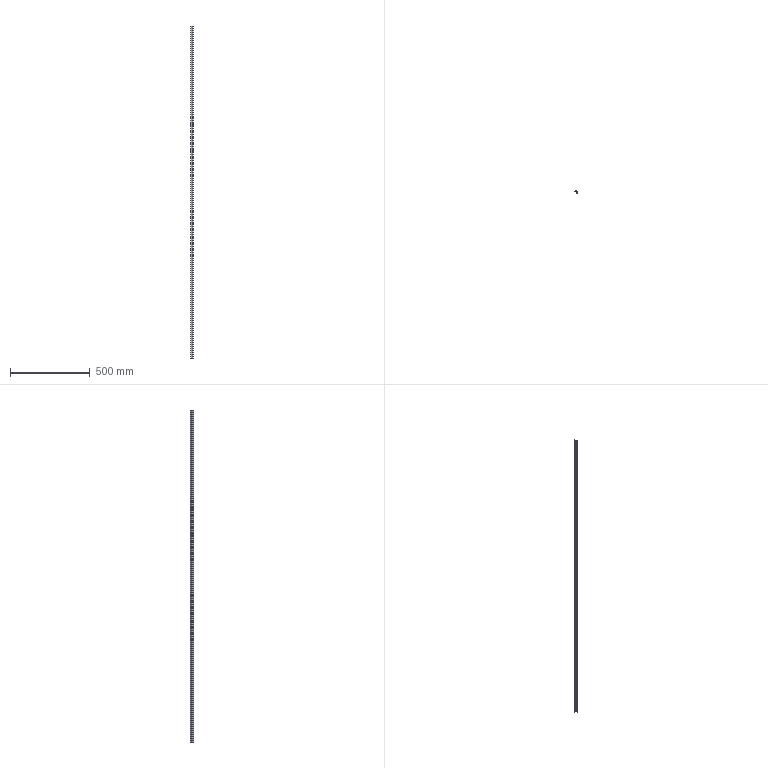Part | SolidWorks | features BaseBody 1, ICE 1, MoveFace 1 | 1 solid | 27 faces | box 14 x 20.3 x 2084 mm | volume 106108 mm3 | plane 20 | cylinder 7 | commonest cylinder face diameters 0.387 x2 0.8 x2 0.4 x1 20 x1 22 x1
STEP:
#1=CARTESIAN_POINT('',(-5.304,-0.625,200.));
#2=VERTEX_POINT('',#1);
#3=CARTESIAN_POINT('',(-5.449,-0.8125,200.));
#4=VERTEX_POINT('',#3);
#5=CARTESIAN_POINT('',(-5.255,-0.8125,200.));
#6=DIRECTION('',(0.,0.,1.));
#7=DIRECTION('',(-1.,0.,0.));
#8=AXIS2_PLACEMENT_3D('',#5,#6,#7);
#9=CIRCLE('',#8,0.1937);
#10=EDGE_CURVE('',#2,#4,#9,.T.);
#11=ORIENTED_EDGE('',*,*,#10,.T.);
#12=CARTESIAN_POINT('',(-5.449,-0.8125,-1884.));
#13=VERTEX_POINT('',#12);
#14=CARTESIAN_POINT('',(-5.449,-0.8125,230.));
#15=DIRECTION('',(0.,0.,-1.));
#16=VECTOR('',#15,1000.);
#17=LINE('',#14,#16);
#18=EDGE_CURVE('',#4,#13,#17,.T.);
#19=ORIENTED_EDGE('',*,*,#18,.T.);
#20=CARTESIAN_POINT('',(-5.304,-0.625,-1884.));
#21=VERTEX_POINT('',#20);
#22=CARTESIAN_POINT('',(-5.255,-0.8125,-1884.));
#23=DIRECTION('',(0.,0.,-1.));
#24=DIRECTION('',(1.,0.,0.));
#25=AXIS2_PLACEMENT_3D('',#22,#23,#24);
#26=CIRCLE('',#25,0.1937);
#27=EDGE_CURVE('',#13,#21,#26,.T.);
#28=ORIENTED_EDGE('',*,*,#27,.T.);
#29=CARTESIAN_POINT('',(-5.304,-0.625,230.));
#30=DIRECTION('',(0.,0.,-1.));
#31=VECTOR('',#30,1000.);
#32=LINE('',#29,#31);
#33=EDGE_CURVE('',#2,#21,#32,.T.);
#34=ORIENTED_EDGE('',*,*,#33,.F.);
#35=EDGE_LOOP('',(#11,#19,#28,#34));
#36=FACE_OUTER_BOUND('',#35,.T.);
#37=CARTESIAN_POINT('',(-5.255,-0.8125,230.));
#38=DIRECTION('',(0.,0.,-1.));
#39=DIRECTION('',(-1.,0.,0.));
#40=AXIS2_PLACEMENT_3D('',#37,#38,#39);
#41=CYLINDRICAL_SURFACE('',#40,0.1937);
#42=ADVANCED_FACE('',(#36),#41,.F.);
#43=CARTESIAN_POINT('',(5.,-1.,-1884.));
#44=VERTEX_POINT('',#43);
#45=CARTESIAN_POINT('',(5.,-14.3,-1884.));
#46=VERTEX_POINT('',#45);
#47=CARTESIAN_POINT('',(5.,29.623,-1884.));
#48=DIRECTION('',(0.,-1.,0.));
#49=VECTOR('',#48,1000.);
#50=LINE('',#47,#49);
#51=EDGE_CURVE('',#44,#46,#50,.T.);
#52=ORIENTED_EDGE('',*,*,#51,.F.);
#53=CARTESIAN_POINT('',(5.,-1.,200.));
#54=VERTEX_POINT('',#53);
#55=CARTESIAN_POINT('',(5.,-1.,230.));
#56=DIRECTION('',(0.,0.,-1.));
#57=VECTOR('',#56,1000.);
#58=LINE('',#55,#57);
#59=EDGE_CURVE('',#54,#44,#58,.T.);
#60=ORIENTED_EDGE('',*,*,#59,.F.);
#61=CARTESIAN_POINT('',(5.,-14.3,200.));
#62=VERTEX_POINT('',#61);
#63=CARTESIAN_POINT('',(5.,-14.3,200.));
#64=DIRECTION('',(0.,1.,0.));
#65=VECTOR('',#64,1000.);
#66=LINE('',#63,#65);
#67=EDGE_CURVE('',#62,#54,#66,.T.);
#68=ORIENTED_EDGE('',*,*,#67,.F.);
#69=CARTESIAN_POINT('',(5.,-14.3,230.));
#70=DIRECTION('',(0.,0.,1.));
#71=VECTOR('',#70,1000.);
#72=LINE('',#69,#71);
#73=EDGE_CURVE('',#46,#62,#72,.T.);
#74=ORIENTED_EDGE('',*,*,#73,.F.);
#75=EDGE_LOOP('',(#52,#60,#68,#74));
#76=FACE_OUTER_BOUND('',#75,.T.);
#77=CARTESIAN_POINT('',(5.,-14.3,230.));
#78=DIRECTION('',(-1.,0.,0.));
#79=DIRECTION('',(0.,0.,1.));
#80=AXIS2_PLACEMENT_3D('',#77,#78,#79);
#81=PLANE('',#80);
#82=ADVANCED_FACE('',(#76),#81,.F.);
#83=CARTESIAN_POINT('',(-9.,-2.,-1884.));
#84=VERTEX_POINT('',#83);
#85=CARTESIAN_POINT('',(-9.,-2.,200.));
#86=VERTEX_POINT('',#85);
#87=CARTESIAN_POINT('',(-9.,-2.,230.));
#88=DIRECTION('',(0.,0.,1.));
#89=VECTOR('',#88,1000.);
#90=LINE('',#87,#89);
#91=EDGE_CURVE('',#84,#86,#90,.T.);
#92=ORIENTED_EDGE('',*,*,#91,.F.);
#93=CARTESIAN_POINT('',(0.9,-2.,-1884.));
#94=VERTEX_POINT('',#93);
#95=CARTESIAN_POINT('',(5.,-2.,-1884.));
#96=DIRECTION('',(-1.,0.,0.));
#97=VECTOR('',#96,1000.);
#98=LINE('',#95,#97);
#99=EDGE_CURVE('',#94,#84,#98,.T.);
#100=ORIENTED_EDGE('',*,*,#99,.F.);
#101=CARTESIAN_POINT('',(0.9,-2.,200.));
#102=VERTEX_POINT('',#101);
#103=CARTESIAN_POINT('',(0.9,-2.,230.));
#104=DIRECTION('',(0.,0.,-1.));
#105=VECTOR('',#104,1000.);
#106=LINE('',#103,#105);
#107=EDGE_CURVE('',#102,#94,#106,.T.);
#108=ORIENTED_EDGE('',*,*,#107,.F.);
#109=CARTESIAN_POINT('',(5.,-2.,200.));
#110=DIRECTION('',(1.,0.,0.));
#111=VECTOR('',#110,1000.);
#112=LINE('',#109,#111);
#113=EDGE_CURVE('',#86,#102,#112,.T.);
#114=ORIENTED_EDGE('',*,*,#113,.F.);
#115=EDGE_LOOP('',(#92,#100,#108,#114));
#116=FACE_OUTER_BOUND('',#115,.T.);
#117=CARTESIAN_POINT('',(-9.,-2.,230.));
#118=DIRECTION('',(0.,1.,0.));
#119=DIRECTION('',(0.,0.,1.));
#120=AXIS2_PLACEMENT_3D('',#117,#118,#119);
#121=PLANE('',#120);
#122=ADVANCED_FACE('',(#116),#121,.F.);
#123=CARTESIAN_POINT('',(4.,-6.,200.));
#124=VERTEX_POINT('',#123);
#125=CARTESIAN_POINT('',(4.,-3.,200.));
#126=VERTEX_POINT('',#125);
#127=CARTESIAN_POINT('',(4.,29.623,200.));
#128=DIRECTION('',(0.,1.,0.));
#129=VECTOR('',#128,1000.);
#130=LINE('',#127,#129);
#131=EDGE_CURVE('',#124,#126,#130,.T.);
#132=ORIENTED_EDGE('',*,*,#131,.F.);
#133=CARTESIAN_POINT('',(1.,-6.,200.));
#134=VERTEX_POINT('',#133);
#135=CARTESIAN_POINT('',(5.,-6.,200.));
#136=DIRECTION('',(1.,0.,0.));
#137=VECTOR('',#136,1000.);
#138=LINE('',#135,#137);
#139=EDGE_CURVE('',#134,#124,#138,.T.);
#140=ORIENTED_EDGE('',*,*,#139,.F.);
#141=CARTESIAN_POINT('',(1.,-6.7,200.));
#142=VERTEX_POINT('',#141);
#143=CARTESIAN_POINT('',(1.,-6.,200.));
#144=DIRECTION('',(0.,-1.,0.));
#145=VECTOR('',#144,1000.);
#146=LINE('',#143,#145);
#147=EDGE_CURVE('',#134,#142,#146,.T.);
#148=ORIENTED_EDGE('',*,*,#147,.T.);
#149=CARTESIAN_POINT('',(-1.7,-6.7,200.));
#150=VERTEX_POINT('',#149);
#151=CARTESIAN_POINT('',(5.,-6.7,200.));
#152=DIRECTION('',(1.,0.,0.));
#153=VECTOR('',#152,1000.);
#154=LINE('',#151,#153);
#155=EDGE_CURVE('',#150,#142,#154,.T.);
#156=ORIENTED_EDGE('',*,*,#155,.F.);
#157=CARTESIAN_POINT('',(-1.7,-7.7,200.));
#158=VERTEX_POINT('',#157);
#159=CARTESIAN_POINT('',(-1.7,-6.7,200.));
#160=DIRECTION('',(0.,-1.,0.));
#161=VECTOR('',#160,1000.);
#162=LINE('',#159,#161);
#163=EDGE_CURVE('',#150,#158,#162,.T.);
#164=ORIENTED_EDGE('',*,*,#163,.T.);
#165=CARTESIAN_POINT('',(4.,-7.7,200.));
#166=VERTEX_POINT('',#165);
#167=CARTESIAN_POINT('',(5.,-7.7,200.));
#168=DIRECTION('',(-1.,0.,0.));
#169=VECTOR('',#168,1000.);
#170=LINE('',#167,#169);
#171=EDGE_CURVE('',#166,#158,#170,.T.);
#172=ORIENTED_EDGE('',*,*,#171,.F.);
#173=CARTESIAN_POINT('',(4.,-14.3,200.));
#174=VERTEX_POINT('',#173);
#175=CARTESIAN_POINT('',(4.,29.623,200.));
#176=DIRECTION('',(0.,1.,0.));
#177=VECTOR('',#176,1000.);
#178=LINE('',#175,#177);
#179=EDGE_CURVE('',#174,#166,#178,.T.);
#180=ORIENTED_EDGE('',*,*,#179,.F.);
#181=CARTESIAN_POINT('',(5.,-14.3,200.));
#182=DIRECTION('',(-1.,0.,0.));
#183=VECTOR('',#182,1000.);
#184=LINE('',#181,#183);
#185=EDGE_CURVE('',#62,#174,#184,.T.);
#186=ORIENTED_EDGE('',*,*,#185,.F.);
#187=ORIENTED_EDGE('',*,*,#67,.T.);
#188=CARTESIAN_POINT('',(-5.207,-1.,200.));
#189=VERTEX_POINT('',#188);
#190=CARTESIAN_POINT('',(5.,-1.,200.));
#191=DIRECTION('',(1.,0.,0.));
#192=VECTOR('',#191,1000.);
#193=LINE('',#190,#192);
#194=EDGE_CURVE('',#189,#54,#193,.T.);
#195=ORIENTED_EDGE('',*,*,#194,.F.);
#196=CARTESIAN_POINT('',(-5.255,-0.8125,200.));
#197=DIRECTION('',(0.,0.,1.));
#198=DIRECTION('',(-1.,0.,0.));
#199=AXIS2_PLACEMENT_3D('',#196,#197,#198);
#200=CIRCLE('',#199,0.1937);
#201=EDGE_CURVE('',#4,#189,#200,.T.);
#202=ORIENTED_EDGE('',*,*,#201,.F.);
#203=ORIENTED_EDGE('',*,*,#10,.F.);
#204=CARTESIAN_POINT('',(-1.368,3.063,200.));
#205=VERTEX_POINT('',#204);
#206=CARTESIAN_POINT('',(-10.628,9.,200.));
#207=DIRECTION('',(0.,0.,1.));
#208=DIRECTION('',(-1.,0.,0.));
#209=AXIS2_PLACEMENT_3D('',#206,#207,#208);
#210=CIRCLE('',#209,11.);
#211=EDGE_CURVE('',#2,#205,#210,.T.);
#212=ORIENTED_EDGE('',*,*,#211,.T.);
#213=CARTESIAN_POINT('',(-1.,2.955,200.));
#214=VERTEX_POINT('',#213);
#215=CARTESIAN_POINT('',(-1.2,2.955,200.));
#216=DIRECTION('',(0.,0.,1.));
#217=DIRECTION('',(-1.,0.,0.));
#218=AXIS2_PLACEMENT_3D('',#215,#216,#217);
#219=CIRCLE('',#218,0.2);
#220=EDGE_CURVE('',#214,#205,#219,.T.);
#221=ORIENTED_EDGE('',*,*,#220,.F.);
#222=CARTESIAN_POINT('',(-1.,1.5,200.));
#223=VERTEX_POINT('',#222);
#224=CARTESIAN_POINT('',(-1.,2.955,200.));
#225=DIRECTION('',(0.,1.,0.));
#226=VECTOR('',#225,1000.);
#227=LINE('',#224,#226);
#228=EDGE_CURVE('',#223,#214,#227,.T.);
#229=ORIENTED_EDGE('',*,*,#228,.F.);
#230=CARTESIAN_POINT('',(0.,1.5,200.));
#231=VERTEX_POINT('',#230);
#232=CARTESIAN_POINT('',(-1.,1.5,200.));
#233=DIRECTION('',(-1.,0.,0.));
#234=VECTOR('',#233,1000.);
#235=LINE('',#232,#234);
#236=EDGE_CURVE('',#231,#223,#235,.T.);
#237=ORIENTED_EDGE('',*,*,#236,.F.);
#238=CARTESIAN_POINT('',(0.,6.,200.));
#239=VERTEX_POINT('',#238);
#240=CARTESIAN_POINT('',(0.,1.5,200.));
#241=DIRECTION('',(0.,-1.,0.));
#242=VECTOR('',#241,1000.);
#243=LINE('',#240,#242);
#244=EDGE_CURVE('',#239,#231,#243,.T.);
#245=ORIENTED_EDGE('',*,*,#244,.F.);
#246=CARTESIAN_POINT('',(-0.8,6.,200.));
#247=VERTEX_POINT('',#246);
#248=CARTESIAN_POINT('',(0.,6.,200.));
#249=DIRECTION('',(1.,0.,0.));
#250=VECTOR('',#249,1000.);
#251=LINE('',#248,#250);
#252=EDGE_CURVE('',#247,#239,#251,.T.);
#253=ORIENTED_EDGE('',*,*,#252,.F.);
#254=CARTESIAN_POINT('',(-1.178,5.731,200.));
#255=VERTEX_POINT('',#254);
#256=CARTESIAN_POINT('',(-0.8,5.6,200.));
#257=DIRECTION('',(0.,0.,1.));
#258=DIRECTION('',(-1.,0.,0.));
#259=AXIS2_PLACEMENT_3D('',#256,#257,#258);
#260=CIRCLE('',#259,0.4);
#261=EDGE_CURVE('',#247,#255,#260,.T.);
#262=ORIENTED_EDGE('',*,*,#261,.T.);
#263=CARTESIAN_POINT('',(-8.678,-0.8077,200.));
#264=VERTEX_POINT('',#263);
#265=CARTESIAN_POINT('',(-10.628,9.,200.));
#266=DIRECTION('',(0.,0.,1.));
#267=DIRECTION('',(-1.,0.,0.));
#268=AXIS2_PLACEMENT_3D('',#265,#266,#267);
#269=CIRCLE('',#268,10.);
#270=EDGE_CURVE('',#264,#255,#269,.T.);
#271=ORIENTED_EDGE('',*,*,#270,.F.);
#272=CARTESIAN_POINT('',(-9.,-1.2,200.));
#273=VERTEX_POINT('',#272);
#274=CARTESIAN_POINT('',(-8.6,-1.2,200.));
#275=DIRECTION('',(0.,0.,1.));
#276=DIRECTION('',(-1.,0.,0.));
#277=AXIS2_PLACEMENT_3D('',#274,#275,#276);
#278=CIRCLE('',#277,0.4);
#279=EDGE_CURVE('',#264,#273,#278,.T.);
#280=ORIENTED_EDGE('',*,*,#279,.T.);
#281=CARTESIAN_POINT('',(-9.,8.,200.));
#282=DIRECTION('',(0.,-1.,0.));
#283=VECTOR('',#282,1000.);
#284=LINE('',#281,#283);
#285=EDGE_CURVE('',#273,#86,#284,.T.);
#286=ORIENTED_EDGE('',*,*,#285,.T.);
#287=ORIENTED_EDGE('',*,*,#113,.T.);
#288=CARTESIAN_POINT('',(0.9,-3.,200.));
#289=VERTEX_POINT('',#288);
#290=CARTESIAN_POINT('',(0.9,29.623,200.));
#291=DIRECTION('',(0.,1.,0.));
#292=VECTOR('',#291,1000.);
#293=LINE('',#290,#292);
#294=EDGE_CURVE('',#289,#102,#293,.T.);
#295=ORIENTED_EDGE('',*,*,#294,.F.);
#296=CARTESIAN_POINT('',(5.,-3.,200.));
#297=DIRECTION('',(-1.,0.,0.));
#298=VECTOR('',#297,1000.);
#299=LINE('',#296,#298);
#300=EDGE_CURVE('',#126,#289,#299,.T.);
#301=ORIENTED_EDGE('',*,*,#300,.F.);
#302=EDGE_LOOP('',(#132,#140,#148,#156,#164,#172,#180,#186,#187,#195,#202,#203,#212,#221,#229,#237,#245,#253,#262,#271,#280,#286,#287,#295,#301));
#303=FACE_OUTER_BOUND('',#302,.T.);
#304=CARTESIAN_POINT('',(5.,29.623,200.));
#305=DIRECTION('',(0.,0.,-1.));
#306=DIRECTION('',(-1.,0.,0.));
#307=AXIS2_PLACEMENT_3D('',#304,#305,#306);
#308=PLANE('',#307);
#309=ADVANCED_FACE('',(#303),#308,.F.);
#310=ORIENTED_EDGE('',*,*,#185,.T.);
#311=CARTESIAN_POINT('',(4.,-14.3,-1884.));
#312=VERTEX_POINT('',#311);
#313=CARTESIAN_POINT('',(4.,-14.3,230.));
#314=DIRECTION('',(0.,0.,1.));
#315=VECTOR('',#314,1000.);
#316=LINE('',#313,#315);
#317=EDGE_CURVE('',#312,#174,#316,.T.);
#318=ORIENTED_EDGE('',*,*,#317,.F.);
#319=CARTESIAN_POINT('',(5.,-14.3,-1884.));
#320=DIRECTION('',(-1.,0.,0.));
#321=VECTOR('',#320,1000.);
#322=LINE('',#319,#321);
#323=EDGE_CURVE('',#46,#312,#322,.T.);
#324=ORIENTED_EDGE('',*,*,#323,.F.);
#325=ORIENTED_EDGE('',*,*,#73,.T.);
#326=EDGE_LOOP('',(#310,#318,#324,#325));
#327=FACE_OUTER_BOUND('',#326,.T.);
#328=CARTESIAN_POINT('',(4.,-14.3,230.));
#329=DIRECTION('',(0.,1.,0.));
#330=DIRECTION('',(0.,0.,1.));
#331=AXIS2_PLACEMENT_3D('',#328,#329,#330);
#332=PLANE('',#331);
#333=ADVANCED_FACE('',(#327),#332,.F.);
#334=ORIENTED_EDGE('',*,*,#51,.T.);
#335=ORIENTED_EDGE('',*,*,#323,.T.);
#336=CARTESIAN_POINT('',(4.,-7.7,-1884.));
#337=VERTEX_POINT('',#336);
#338=CARTESIAN_POINT('',(4.,-7.7,-1884.));
#339=DIRECTION('',(0.,-1.,0.));
#340=VECTOR('',#339,1000.);
#341=LINE('',#338,#340);
#342=EDGE_CURVE('',#337,#312,#341,.T.);
#343=ORIENTED_EDGE('',*,*,#342,.F.);
#344=CARTESIAN_POINT('',(-1.7,-7.7,-1884.));
#345=VERTEX_POINT('',#344);
#346=CARTESIAN_POINT('',(-1.7,-7.7,-1884.));
#347=DIRECTION('',(1.,0.,0.));
#348=VECTOR('',#347,1000.);
#349=LINE('',#346,#348);
#350=EDGE_CURVE('',#345,#337,#349,.T.);
#351=ORIENTED_EDGE('',*,*,#350,.F.);
#352=CARTESIAN_POINT('',(-1.7,-6.7,-1884.));
#353=VERTEX_POINT('',#352);
#354=CARTESIAN_POINT('',(-1.7,29.623,-1884.));
#355=DIRECTION('',(0.,1.,0.));
#356=VECTOR('',#355,1000.);
#357=LINE('',#354,#356);
#358=EDGE_CURVE('',#345,#353,#357,.T.);
#359=ORIENTED_EDGE('',*,*,#358,.T.);
#360=CARTESIAN_POINT('',(1.,-6.7,-1884.));
#361=VERTEX_POINT('',#360);
#362=CARTESIAN_POINT('',(1.,-6.7,-1884.));
#363=DIRECTION('',(-1.,0.,0.));
#364=VECTOR('',#363,1000.);
#365=LINE('',#362,#364);
#366=EDGE_CURVE('',#361,#353,#365,.T.);
#367=ORIENTED_EDGE('',*,*,#366,.F.);
#368=CARTESIAN_POINT('',(1.,-6.,-1884.));
#369=VERTEX_POINT('',#368);
#370=CARTESIAN_POINT('',(1.,29.623,-1884.));
#371=DIRECTION('',(0.,1.,0.));
#372=VECTOR('',#371,1000.);
#373=LINE('',#370,#372);
#374=EDGE_CURVE('',#361,#369,#373,.T.);
#375=ORIENTED_EDGE('',*,*,#374,.T.);
#376=CARTESIAN_POINT('',(4.,-6.,-1884.));
#377=VERTEX_POINT('',#376);
#378=CARTESIAN_POINT('',(4.,-6.,-1884.));
#379=DIRECTION('',(-1.,0.,0.));
#380=VECTOR('',#379,1000.);
#381=LINE('',#378,#380);
#382=EDGE_CURVE('',#377,#369,#381,.T.);
#383=ORIENTED_EDGE('',*,*,#382,.F.);
#384=CARTESIAN_POINT('',(4.,-3.,-1884.));
#385=VERTEX_POINT('',#384);
#386=CARTESIAN_POINT('',(4.,-3.,-1884.));
#387=DIRECTION('',(0.,-1.,0.));
#388=VECTOR('',#387,1000.);
#389=LINE('',#386,#388);
#390=EDGE_CURVE('',#385,#377,#389,.T.);
#391=ORIENTED_EDGE('',*,*,#390,.F.);
#392=CARTESIAN_POINT('',(0.9,-3.,-1884.));
#393=VERTEX_POINT('',#392);
#394=CARTESIAN_POINT('',(0.9,-3.,-1884.));
#395=DIRECTION('',(1.,0.,0.));
#396=VECTOR('',#395,1000.);
#397=LINE('',#394,#396);
#398=EDGE_CURVE('',#393,#385,#397,.T.);
#399=ORIENTED_EDGE('',*,*,#398,.F.);
#400=CARTESIAN_POINT('',(0.9,-2.,-1884.));
#401=DIRECTION('',(0.,-1.,0.));
#402=VECTOR('',#401,1000.);
#403=LINE('',#400,#402);
#404=EDGE_CURVE('',#94,#393,#403,.T.);
#405=ORIENTED_EDGE('',*,*,#404,.F.);
#406=ORIENTED_EDGE('',*,*,#99,.T.);
#407=CARTESIAN_POINT('',(-9.,-1.2,-1884.));
#408=VERTEX_POINT('',#407);
#409=CARTESIAN_POINT('',(-9.,-1.2,-1884.));
#410=DIRECTION('',(0.,-1.,0.));
#411=VECTOR('',#410,1000.);
#412=LINE('',#409,#411);
#413=EDGE_CURVE('',#408,#84,#412,.T.);
#414=ORIENTED_EDGE('',*,*,#413,.F.);
#415=CARTESIAN_POINT('',(-8.678,-0.8077,-1884.));
#416=VERTEX_POINT('',#415);
#417=CARTESIAN_POINT('',(-8.6,-1.2,-1884.));
#418=DIRECTION('',(0.,0.,-1.));
#419=DIRECTION('',(1.,0.,0.));
#420=AXIS2_PLACEMENT_3D('',#417,#418,#419);
#421=CIRCLE('',#420,0.4);
#422=EDGE_CURVE('',#408,#416,#421,.T.);
#423=ORIENTED_EDGE('',*,*,#422,.T.);
#424=CARTESIAN_POINT('',(-1.178,5.731,-1884.));
#425=VERTEX_POINT('',#424);
#426=CARTESIAN_POINT('',(-10.628,9.,-1884.));
#427=DIRECTION('',(0.,0.,-1.));
#428=DIRECTION('',(1.,0.,0.));
#429=AXIS2_PLACEMENT_3D('',#426,#427,#428);
#430=CIRCLE('',#429,10.);
#431=EDGE_CURVE('',#425,#416,#430,.T.);
#432=ORIENTED_EDGE('',*,*,#431,.F.);
#433=CARTESIAN_POINT('',(-0.8,6.,-1884.));
#434=VERTEX_POINT('',#433);
#435=CARTESIAN_POINT('',(-0.8,5.6,-1884.));
#436=DIRECTION('',(0.,0.,-1.));
#437=DIRECTION('',(1.,0.,0.));
#438=AXIS2_PLACEMENT_3D('',#435,#436,#437);
#439=CIRCLE('',#438,0.4);
#440=EDGE_CURVE('',#425,#434,#439,.T.);
#441=ORIENTED_EDGE('',*,*,#440,.T.);
#442=CARTESIAN_POINT('',(0.,6.,-1884.));
#443=VERTEX_POINT('',#442);
#444=CARTESIAN_POINT('',(0.,6.,-1884.));
#445=DIRECTION('',(-1.,0.,0.));
#446=VECTOR('',#445,1000.);
#447=LINE('',#444,#446);
#448=EDGE_CURVE('',#443,#434,#447,.T.);
#449=ORIENTED_EDGE('',*,*,#448,.F.);
#450=CARTESIAN_POINT('',(0.,1.5,-1884.));
#451=VERTEX_POINT('',#450);
#452=CARTESIAN_POINT('',(0.,1.5,-1884.));
#453=DIRECTION('',(0.,1.,0.));
#454=VECTOR('',#453,1000.);
#455=LINE('',#452,#454);
#456=EDGE_CURVE('',#451,#443,#455,.T.);
#457=ORIENTED_EDGE('',*,*,#456,.F.);
#458=CARTESIAN_POINT('',(-1.,1.5,-1884.));
#459=VERTEX_POINT('',#458);
#460=CARTESIAN_POINT('',(-1.,1.5,-1884.));
#461=DIRECTION('',(1.,0.,0.));
#462=VECTOR('',#461,1000.);
#463=LINE('',#460,#462);
#464=EDGE_CURVE('',#459,#451,#463,.T.);
#465=ORIENTED_EDGE('',*,*,#464,.F.);
#466=CARTESIAN_POINT('',(-1.,2.955,-1884.));
#467=VERTEX_POINT('',#466);
#468=CARTESIAN_POINT('',(-1.,2.955,-1884.));
#469=DIRECTION('',(0.,-1.,0.));
#470=VECTOR('',#469,1000.);
#471=LINE('',#468,#470);
#472=EDGE_CURVE('',#467,#459,#471,.T.);
#473=ORIENTED_EDGE('',*,*,#472,.F.);
#474=CARTESIAN_POINT('',(-1.368,3.063,-1884.));
#475=VERTEX_POINT('',#474);
#476=CARTESIAN_POINT('',(-1.2,2.955,-1884.));
#477=DIRECTION('',(0.,0.,-1.));
#478=DIRECTION('',(1.,0.,0.));
#479=AXIS2_PLACEMENT_3D('',#476,#477,#478);
#480=CIRCLE('',#479,0.2);
#481=EDGE_CURVE('',#475,#467,#480,.T.);
#482=ORIENTED_EDGE('',*,*,#481,.F.);
#483=CARTESIAN_POINT('',(-10.628,9.,-1884.));
#484=DIRECTION('',(0.,0.,-1.));
#485=DIRECTION('',(1.,0.,0.));
#486=AXIS2_PLACEMENT_3D('',#483,#484,#485);
#487=CIRCLE('',#486,11.);
#488=EDGE_CURVE('',#475,#21,#487,.T.);
#489=ORIENTED_EDGE('',*,*,#488,.T.);
#490=ORIENTED_EDGE('',*,*,#27,.F.);
#491=CARTESIAN_POINT('',(-5.207,-1.,-1884.));
#492=VERTEX_POINT('',#491);
#493=CARTESIAN_POINT('',(-5.255,-0.8125,-1884.));
#494=DIRECTION('',(0.,0.,-1.));
#495=DIRECTION('',(1.,0.,0.));
#496=AXIS2_PLACEMENT_3D('',#493,#494,#495);
#497=CIRCLE('',#496,0.1937);
#498=EDGE_CURVE('',#492,#13,#497,.T.);
#499=ORIENTED_EDGE('',*,*,#498,.F.);
#500=CARTESIAN_POINT('',(5.,-1.,-1884.));
#501=DIRECTION('',(-1.,0.,0.));
#502=VECTOR('',#501,1000.);
#503=LINE('',#500,#502);
#504=EDGE_CURVE('',#44,#492,#503,.T.);
#505=ORIENTED_EDGE('',*,*,#504,.F.);
#506=EDGE_LOOP('',(#334,#335,#343,#351,#359,#367,#375,#383,#391,#399,#405,#406,#414,#423,#432,#441,#449,#457,#465,#473,#482,#489,#490,#499,#505));
#507=FACE_OUTER_BOUND('',#506,.T.);
#508=CARTESIAN_POINT('',(5.,29.623,-1884.));
#509=DIRECTION('',(0.,0.,1.));
#510=DIRECTION('',(1.,0.,0.));
#511=AXIS2_PLACEMENT_3D('',#508,#509,#510);
#512=PLANE('',#511);
#513=ADVANCED_FACE('',(#507),#512,.F.);
#514=ORIENTED_EDGE('',*,*,#59,.T.);
#515=ORIENTED_EDGE('',*,*,#504,.T.);
#516=CARTESIAN_POINT('',(-5.207,-1.,230.));
#517=DIRECTION('',(0.,0.,-1.));
#518=VECTOR('',#517,1000.);
#519=LINE('',#516,#518);
#520=EDGE_CURVE('',#189,#492,#519,.T.);
#521=ORIENTED_EDGE('',*,*,#520,.F.);
#522=ORIENTED_EDGE('',*,*,#194,.T.);
#523=EDGE_LOOP('',(#514,#515,#521,#522));
#524=FACE_OUTER_BOUND('',#523,.T.);
#525=CARTESIAN_POINT('',(5.,-1.,230.));
#526=DIRECTION('',(0.,-1.,0.));
#527=DIRECTION('',(0.,0.,-1.));
#528=AXIS2_PLACEMENT_3D('',#525,#526,#527);
#529=PLANE('',#528);
#530=ADVANCED_FACE('',(#524),#529,.F.);
#531=CARTESIAN_POINT('',(-9.,-1.2,230.));
#532=DIRECTION('',(0.,0.,1.));
#533=VECTOR('',#532,1000.);
#534=LINE('',#531,#533);
#535=EDGE_CURVE('',#408,#273,#534,.T.);
#536=ORIENTED_EDGE('',*,*,#535,.F.);
#537=ORIENTED_EDGE('',*,*,#413,.T.);
#538=ORIENTED_EDGE('',*,*,#91,.T.);
#539=ORIENTED_EDGE('',*,*,#285,.F.);
#540=EDGE_LOOP('',(#536,#537,#538,#539));
#541=FACE_OUTER_BOUND('',#540,.T.);
#542=CARTESIAN_POINT('',(-9.,-1.2,230.));
#543=DIRECTION('',(1.,0.,0.));
#544=DIRECTION('',(0.,0.,-1.));
#545=AXIS2_PLACEMENT_3D('',#542,#543,#544);
#546=PLANE('',#545);
#547=ADVANCED_FACE('',(#541),#546,.F.);
#548=ORIENTED_EDGE('',*,*,#294,.T.);
#549=ORIENTED_EDGE('',*,*,#107,.T.);
#550=ORIENTED_EDGE('',*,*,#404,.T.);
#551=CARTESIAN_POINT('',(0.9,-3.,230.));
#552=DIRECTION('',(0.,0.,-1.));
#553=VECTOR('',#552,1000.);
#554=LINE('',#551,#553);
#555=EDGE_CURVE('',#289,#393,#554,.T.);
#556=ORIENTED_EDGE('',*,*,#555,.F.);
#557=EDGE_LOOP('',(#548,#549,#550,#556));
#558=FACE_OUTER_BOUND('',#557,.T.);
#559=CARTESIAN_POINT('',(0.9,-2.,230.));
#560=DIRECTION('',(1.,0.,0.));
#561=DIRECTION('',(0.,0.,-1.));
#562=AXIS2_PLACEMENT_3D('',#559,#560,#561);
#563=PLANE('',#562);
#564=ADVANCED_FACE('',(#558),#563,.F.);
#565=ORIENTED_EDGE('',*,*,#300,.T.);
#566=ORIENTED_EDGE('',*,*,#555,.T.);
#567=ORIENTED_EDGE('',*,*,#398,.T.);
#568=CARTESIAN_POINT('',(4.,-3.,230.));
#569=DIRECTION('',(0.,0.,-1.));
#570=VECTOR('',#569,1000.);
#571=LINE('',#568,#570);
#572=EDGE_CURVE('',#126,#385,#571,.T.);
#573=ORIENTED_EDGE('',*,*,#572,.F.);
#574=EDGE_LOOP('',(#565,#566,#567,#573));
#575=FACE_OUTER_BOUND('',#574,.T.);
#576=CARTESIAN_POINT('',(0.9,-3.,230.));
#577=DIRECTION('',(0.,1.,0.));
#578=DIRECTION('',(0.,0.,1.));
#579=AXIS2_PLACEMENT_3D('',#576,#577,#578);
#580=PLANE('',#579);
#581=ADVANCED_FACE('',(#575),#580,.F.);
#582=ORIENTED_EDGE('',*,*,#131,.T.);
#583=ORIENTED_EDGE('',*,*,#572,.T.);
#584=ORIENTED_EDGE('',*,*,#390,.T.);
#585=CARTESIAN_POINT('',(4.,-6.,230.));
#586=DIRECTION('',(0.,0.,-1.));
#587=VECTOR('',#586,1000.);
#588=LINE('',#585,#587);
#589=EDGE_CURVE('',#124,#377,#588,.T.);
#590=ORIENTED_EDGE('',*,*,#589,.F.);
#591=EDGE_LOOP('',(#582,#583,#584,#590));
#592=FACE_OUTER_BOUND('',#591,.T.);
#593=CARTESIAN_POINT('',(4.,-3.,230.));
#594=DIRECTION('',(1.,0.,0.));
#595=DIRECTION('',(0.,0.,-1.));
#596=AXIS2_PLACEMENT_3D('',#593,#594,#595);
#597=PLANE('',#596);
#598=ADVANCED_FACE('',(#592),#597,.F.);
#599=ORIENTED_EDGE('',*,*,#139,.T.);
#600=ORIENTED_EDGE('',*,*,#589,.T.);
#601=ORIENTED_EDGE('',*,*,#382,.T.);
#602=CARTESIAN_POINT('',(1.,-6.,230.));
#603=DIRECTION('',(0.,0.,-1.));
#604=VECTOR('',#603,1000.);
#605=LINE('',#602,#604);
#606=EDGE_CURVE('',#134,#369,#605,.T.);
#607=ORIENTED_EDGE('',*,*,#606,.F.);
#608=EDGE_LOOP('',(#599,#600,#601,#607));
#609=FACE_OUTER_BOUND('',#608,.T.);
#610=CARTESIAN_POINT('',(4.,-6.,230.));
#611=DIRECTION('',(0.,-1.,0.));
#612=DIRECTION('',(0.,0.,-1.));
#613=AXIS2_PLACEMENT_3D('',#610,#611,#612);
#614=PLANE('',#613);
#615=ADVANCED_FACE('',(#609),#614,.F.);
#616=ORIENTED_EDGE('',*,*,#155,.T.);
#617=CARTESIAN_POINT('',(1.,-6.7,230.));
#618=DIRECTION('',(0.,0.,1.));
#619=VECTOR('',#618,1000.);
#620=LINE('',#617,#619);
#621=EDGE_CURVE('',#361,#142,#620,.T.);
#622=ORIENTED_EDGE('',*,*,#621,.F.);
#623=ORIENTED_EDGE('',*,*,#366,.T.);
#624=CARTESIAN_POINT('',(-1.7,-6.7,230.));
#625=DIRECTION('',(0.,0.,-1.));
#626=VECTOR('',#625,1000.);
#627=LINE('',#624,#626);
#628=EDGE_CURVE('',#150,#353,#627,.T.);
#629=ORIENTED_EDGE('',*,*,#628,.F.);
#630=EDGE_LOOP('',(#616,#622,#623,#629));
#631=FACE_OUTER_BOUND('',#630,.T.);
#632=CARTESIAN_POINT('',(1.,-6.7,230.));
#633=DIRECTION('',(0.,-1.,0.));
#634=DIRECTION('',(0.,0.,-1.));
#635=AXIS2_PLACEMENT_3D('',#632,#633,#634);
#636=PLANE('',#635);
#637=ADVANCED_FACE('',(#631),#636,.F.);
#638=ORIENTED_EDGE('',*,*,#171,.T.);
#639=CARTESIAN_POINT('',(-1.7,-7.7,230.));
#640=DIRECTION('',(0.,0.,1.));
#641=VECTOR('',#640,1000.);
#642=LINE('',#639,#641);
#643=EDGE_CURVE('',#345,#158,#642,.T.);
#644=ORIENTED_EDGE('',*,*,#643,.F.);
#645=ORIENTED_EDGE('',*,*,#350,.T.);
#646=CARTESIAN_POINT('',(4.,-7.7,230.));
#647=DIRECTION('',(0.,0.,-1.));
#648=VECTOR('',#647,1000.);
#649=LINE('',#646,#648);
#650=EDGE_CURVE('',#166,#337,#649,.T.);
#651=ORIENTED_EDGE('',*,*,#650,.F.);
#652=EDGE_LOOP('',(#638,#644,#645,#651));
#653=FACE_OUTER_BOUND('',#652,.T.);
#654=CARTESIAN_POINT('',(-1.7,-7.7,230.));
#655=DIRECTION('',(0.,1.,0.));
#656=DIRECTION('',(0.,0.,1.));
#657=AXIS2_PLACEMENT_3D('',#654,#655,#656);
#658=PLANE('',#657);
#659=ADVANCED_FACE('',(#653),#658,.F.);
#660=ORIENTED_EDGE('',*,*,#179,.T.);
#661=ORIENTED_EDGE('',*,*,#650,.T.);
#662=ORIENTED_EDGE('',*,*,#342,.T.);
#663=ORIENTED_EDGE('',*,*,#317,.T.);
#664=EDGE_LOOP('',(#660,#661,#662,#663));
#665=FACE_OUTER_BOUND('',#664,.T.);
#666=CARTESIAN_POINT('',(4.,-7.7,230.));
#667=DIRECTION('',(1.,0.,0.));
#668=DIRECTION('',(0.,0.,-1.));
#669=AXIS2_PLACEMENT_3D('',#666,#667,#668);
#670=PLANE('',#669);
#671=ADVANCED_FACE('',(#665),#670,.F.);
#672=ORIENTED_EDGE('',*,*,#18,.F.);
#673=ORIENTED_EDGE('',*,*,#201,.T.);
#674=ORIENTED_EDGE('',*,*,#520,.T.);
#675=ORIENTED_EDGE('',*,*,#498,.T.);
#676=EDGE_LOOP('',(#672,#673,#674,#675));
#677=FACE_OUTER_BOUND('',#676,.T.);
#678=CARTESIAN_POINT('',(-5.255,-0.8125,230.));
#679=DIRECTION('',(0.,0.,-1.));
#680=DIRECTION('',(-1.,0.,0.));
#681=AXIS2_PLACEMENT_3D('',#678,#679,#680);
#682=CYLINDRICAL_SURFACE('',#681,0.1937);
#683=ADVANCED_FACE('',(#677),#682,.F.);
#684=CARTESIAN_POINT('',(-1.,2.955,230.));
#685=DIRECTION('',(0.,0.,1.));
#686=VECTOR('',#685,1000.);
#687=LINE('',#684,#686);
#688=EDGE_CURVE('',#467,#214,#687,.T.);
#689=ORIENTED_EDGE('',*,*,#688,.F.);
#690=ORIENTED_EDGE('',*,*,#472,.T.);
#691=CARTESIAN_POINT('',(-1.,1.5,230.));
#692=DIRECTION('',(0.,0.,-1.));
#693=VECTOR('',#692,1000.);
#694=LINE('',#691,#693);
#695=EDGE_CURVE('',#223,#459,#694,.T.);
#696=ORIENTED_EDGE('',*,*,#695,.F.);
#697=ORIENTED_EDGE('',*,*,#228,.T.);
#698=EDGE_LOOP('',(#689,#690,#696,#697));
#699=FACE_OUTER_BOUND('',#698,.T.);
#700=CARTESIAN_POINT('',(-1.,2.955,230.));
#701=DIRECTION('',(1.,0.,0.));
#702=DIRECTION('',(0.,0.,-1.));
#703=AXIS2_PLACEMENT_3D('',#700,#701,#702);
#704=PLANE('',#703);
#705=ADVANCED_FACE('',(#699),#704,.F.);
#706=ORIENTED_EDGE('',*,*,#488,.F.);
#707=CARTESIAN_POINT('',(-1.368,3.063,230.));
#708=DIRECTION('',(0.,0.,1.));
#709=VECTOR('',#708,1000.);
#710=LINE('',#707,#709);
#711=EDGE_CURVE('',#475,#205,#710,.T.);
#712=ORIENTED_EDGE('',*,*,#711,.T.);
#713=ORIENTED_EDGE('',*,*,#211,.F.);
#714=ORIENTED_EDGE('',*,*,#33,.T.);
#715=EDGE_LOOP('',(#706,#712,#713,#714));
#716=FACE_OUTER_BOUND('',#715,.T.);
#717=CARTESIAN_POINT('',(-10.628,9.,230.));
#718=DIRECTION('',(0.,0.,-1.));
#719=DIRECTION('',(-1.,0.,0.));
#720=AXIS2_PLACEMENT_3D('',#717,#718,#719);
#721=CYLINDRICAL_SURFACE('',#720,11.);
#722=ADVANCED_FACE('',(#716),#721,.T.);
#723=CARTESIAN_POINT('',(-1.178,5.731,230.));
#724=DIRECTION('',(0.,0.,1.));
#725=VECTOR('',#724,1000.);
#726=LINE('',#723,#725);
#727=EDGE_CURVE('',#425,#255,#726,.T.);
#728=ORIENTED_EDGE('',*,*,#727,.F.);
#729=ORIENTED_EDGE('',*,*,#431,.T.);
#730=CARTESIAN_POINT('',(-8.678,-0.8077,230.));
#731=DIRECTION('',(0.,0.,-1.));
#732=VECTOR('',#731,1000.);
#733=LINE('',#730,#732);
#734=EDGE_CURVE('',#264,#416,#733,.T.);
#735=ORIENTED_EDGE('',*,*,#734,.F.);
#736=ORIENTED_EDGE('',*,*,#270,.T.);
#737=EDGE_LOOP('',(#728,#729,#735,#736));
#738=FACE_OUTER_BOUND('',#737,.T.);
#739=CARTESIAN_POINT('',(-10.628,9.,230.));
#740=DIRECTION('',(0.,0.,-1.));
#741=DIRECTION('',(-1.,0.,0.));
#742=AXIS2_PLACEMENT_3D('',#739,#740,#741);
#743=CYLINDRICAL_SURFACE('',#742,10.);
#744=ADVANCED_FACE('',(#738),#743,.F.);
#745=CARTESIAN_POINT('',(0.,1.5,230.));
#746=DIRECTION('',(0.,0.,1.));
#747=VECTOR('',#746,1000.);
#748=LINE('',#745,#747);
#749=EDGE_CURVE('',#451,#231,#748,.T.);
#750=ORIENTED_EDGE('',*,*,#749,.F.);
#751=ORIENTED_EDGE('',*,*,#456,.T.);
#752=CARTESIAN_POINT('',(0.,6.,230.));
#753=DIRECTION('',(0.,0.,-1.));
#754=VECTOR('',#753,1000.);
#755=LINE('',#752,#754);
#756=EDGE_CURVE('',#239,#443,#755,.T.);
#757=ORIENTED_EDGE('',*,*,#756,.F.);
#758=ORIENTED_EDGE('',*,*,#244,.T.);
#759=EDGE_LOOP('',(#750,#751,#757,#758));
#760=FACE_OUTER_BOUND('',#759,.T.);
#761=CARTESIAN_POINT('',(0.,1.5,230.));
#762=DIRECTION('',(-1.,0.,0.));
#763=DIRECTION('',(0.,0.,1.));
#764=AXIS2_PLACEMENT_3D('',#761,#762,#763);
#765=PLANE('',#764);
#766=ADVANCED_FACE('',(#760),#765,.F.);
#767=ORIENTED_EDGE('',*,*,#422,.F.);
#768=ORIENTED_EDGE('',*,*,#535,.T.);
#769=ORIENTED_EDGE('',*,*,#279,.F.);
#770=ORIENTED_EDGE('',*,*,#734,.T.);
#771=EDGE_LOOP('',(#767,#768,#769,#770));
#772=FACE_OUTER_BOUND('',#771,.T.);
#773=CARTESIAN_POINT('',(-8.6,-1.2,230.));
#774=DIRECTION('',(0.,0.,-1.));
#775=DIRECTION('',(-1.,0.,0.));
#776=AXIS2_PLACEMENT_3D('',#773,#774,#775);
#777=CYLINDRICAL_SURFACE('',#776,0.4);
#778=ADVANCED_FACE('',(#772),#777,.T.);
#779=ORIENTED_EDGE('',*,*,#147,.F.);
#780=ORIENTED_EDGE('',*,*,#606,.T.);
#781=ORIENTED_EDGE('',*,*,#374,.F.);
#782=ORIENTED_EDGE('',*,*,#621,.T.);
#783=EDGE_LOOP('',(#779,#780,#781,#782));
#784=FACE_OUTER_BOUND('',#783,.T.);
#785=CARTESIAN_POINT('',(1.,-6.,230.));
#786=DIRECTION('',(1.,0.,0.));
#787=DIRECTION('',(0.,0.,-1.));
#788=AXIS2_PLACEMENT_3D('',#785,#786,#787);
#789=PLANE('',#788);
#790=ADVANCED_FACE('',(#784),#789,.F.);
#791=ORIENTED_EDGE('',*,*,#163,.F.);
#792=ORIENTED_EDGE('',*,*,#628,.T.);
#793=ORIENTED_EDGE('',*,*,#358,.F.);
#794=ORIENTED_EDGE('',*,*,#643,.T.);
#795=EDGE_LOOP('',(#791,#792,#793,#794));
#796=FACE_OUTER_BOUND('',#795,.T.);
#797=CARTESIAN_POINT('',(-1.7,-6.7,230.));
#798=DIRECTION('',(1.,0.,0.));
#799=DIRECTION('',(0.,0.,-1.));
#800=AXIS2_PLACEMENT_3D('',#797,#798,#799);
#801=PLANE('',#800);
#802=ADVANCED_FACE('',(#796),#801,.F.);
#803=ORIENTED_EDGE('',*,*,#711,.F.);
#804=ORIENTED_EDGE('',*,*,#481,.T.);
#805=ORIENTED_EDGE('',*,*,#688,.T.);
#806=ORIENTED_EDGE('',*,*,#220,.T.);
#807=EDGE_LOOP('',(#803,#804,#805,#806));
#808=FACE_OUTER_BOUND('',#807,.T.);
#809=CARTESIAN_POINT('',(-1.2,2.955,230.));
#810=DIRECTION('',(0.,0.,-1.));
#811=DIRECTION('',(-1.,0.,0.));
#812=AXIS2_PLACEMENT_3D('',#809,#810,#811);
#813=CYLINDRICAL_SURFACE('',#812,0.2);
#814=ADVANCED_FACE('',(#808),#813,.F.);
#815=ORIENTED_EDGE('',*,*,#695,.T.);
#816=ORIENTED_EDGE('',*,*,#464,.T.);
#817=ORIENTED_EDGE('',*,*,#749,.T.);
#818=ORIENTED_EDGE('',*,*,#236,.T.);
#819=EDGE_LOOP('',(#815,#816,#817,#818));
#820=FACE_OUTER_BOUND('',#819,.T.);
#821=CARTESIAN_POINT('',(-1.,1.5,230.));
#822=DIRECTION('',(0.,1.,0.));
#823=DIRECTION('',(0.,0.,1.));
#824=AXIS2_PLACEMENT_3D('',#821,#822,#823);
#825=PLANE('',#824);
#826=ADVANCED_FACE('',(#820),#825,.F.);
#827=ORIENTED_EDGE('',*,*,#440,.F.);
#828=ORIENTED_EDGE('',*,*,#727,.T.);
#829=ORIENTED_EDGE('',*,*,#261,.F.);
#830=CARTESIAN_POINT('',(-0.8,6.,230.));
#831=DIRECTION('',(0.,0.,-1.));
#832=VECTOR('',#831,1000.);
#833=LINE('',#830,#832);
#834=EDGE_CURVE('',#247,#434,#833,.T.);
#835=ORIENTED_EDGE('',*,*,#834,.T.);
#836=EDGE_LOOP('',(#827,#828,#829,#835));
#837=FACE_OUTER_BOUND('',#836,.T.);
#838=CARTESIAN_POINT('',(-0.8,5.6,230.));
#839=DIRECTION('',(0.,0.,-1.));
#840=DIRECTION('',(-1.,0.,0.));
#841=AXIS2_PLACEMENT_3D('',#838,#839,#840);
#842=CYLINDRICAL_SURFACE('',#841,0.4);
#843=ADVANCED_FACE('',(#837),#842,.T.);
#844=ORIENTED_EDGE('',*,*,#756,.T.);
#845=ORIENTED_EDGE('',*,*,#448,.T.);
#846=ORIENTED_EDGE('',*,*,#834,.F.);
#847=ORIENTED_EDGE('',*,*,#252,.T.);
#848=EDGE_LOOP('',(#844,#845,#846,#847));
#849=FACE_OUTER_BOUND('',#848,.T.);
#850=CARTESIAN_POINT('',(0.,6.,230.));
#851=DIRECTION('',(0.,-1.,0.));
#852=DIRECTION('',(0.,0.,-1.));
#853=AXIS2_PLACEMENT_3D('',#850,#851,#852);
#854=PLANE('',#853);
#855=ADVANCED_FACE('',(#849),#854,.F.);
#856=CLOSED_SHELL('',(#42,#82,#122,#309,#333,#513,#530,#547,#564,#581,#598,#615,#637,#659,#671,#683,#705,#722,#744,#766,#778,#790,#802,#814,#826,#843,#855));
#857=MANIFOLD_SOLID_BREP('',#856);
#858=CARTESIAN_POINT('',(0.,0.,0.));
#859=DIRECTION('',(0.,0.,1.));
#860=DIRECTION('',(1.,0.,0.));
#861=AXIS2_PLACEMENT_3D('',#858,#859,#860);
#862=(LENGTH_UNIT()NAMED_UNIT(*)SI_UNIT(.MILLI.,.METRE.));
#863=UNCERTAINTY_MEASURE_WITH_UNIT(LENGTH_MEASURE(0.00001),#862,'','');
#864=(NAMED_UNIT(*)PLANE_ANGLE_UNIT()SI_UNIT($,.RADIAN.));
#865=(NAMED_UNIT(*)SI_UNIT($,.STERADIAN.)SOLID_ANGLE_UNIT());
#866=(GEOMETRIC_REPRESENTATION_CONTEXT(3)GLOBAL_UNCERTAINTY_ASSIGNED_CONTEXT((#863))GLOBAL_UNIT_ASSIGNED_CONTEXT((#862,#864,#865))REPRESENTATION_CONTEXT('',''));
#867=ADVANCED_BREP_SHAPE_REPRESENTATION('',(#857,#861),#866);